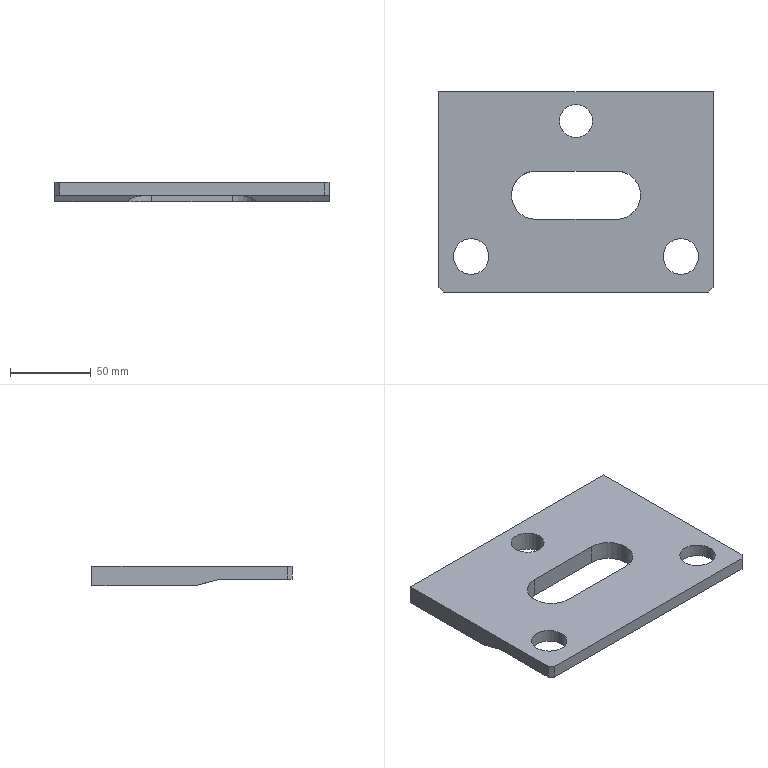Part | STEP file | support plate 31 | 1 solid | 38 faces | box 170 x 124 x 12 mm | volume 181853 mm3 | cylinder 17 | plane 13 | cone 8 | commonest cylinder face diameters 4.2 x8 22 x4 30 x3 20.5 x2